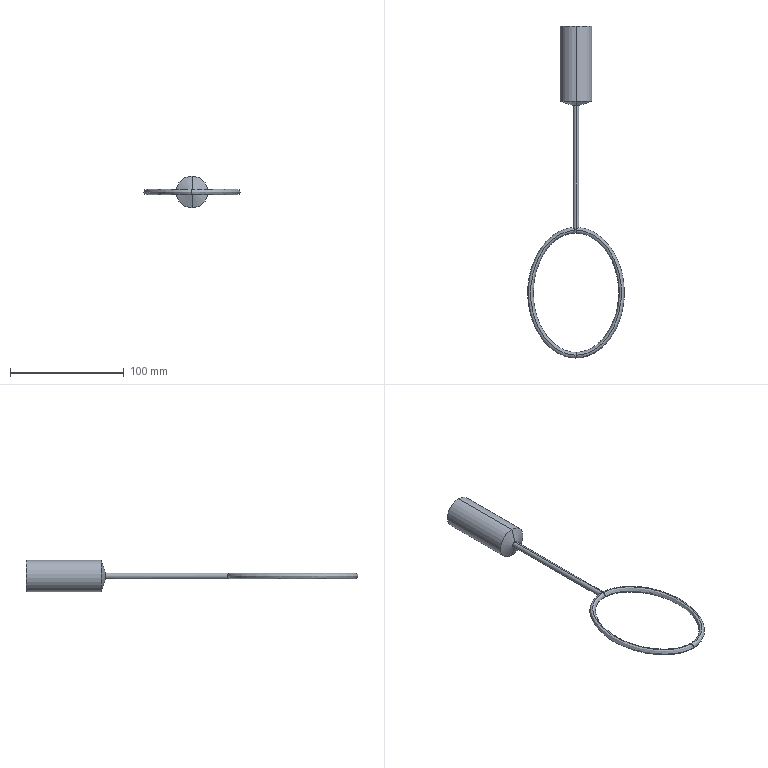Part | SolidWorks | features ICE 2, RevCut 1, Sweep 1 | 1 solid | 11 faces | box 85 x 292.5 x 28 mm | volume 49744 mm3 | spline 4 | cylinder 4 | cone 2 | plane 1 | commonest cylinder face diameters 5 x2 28 x2